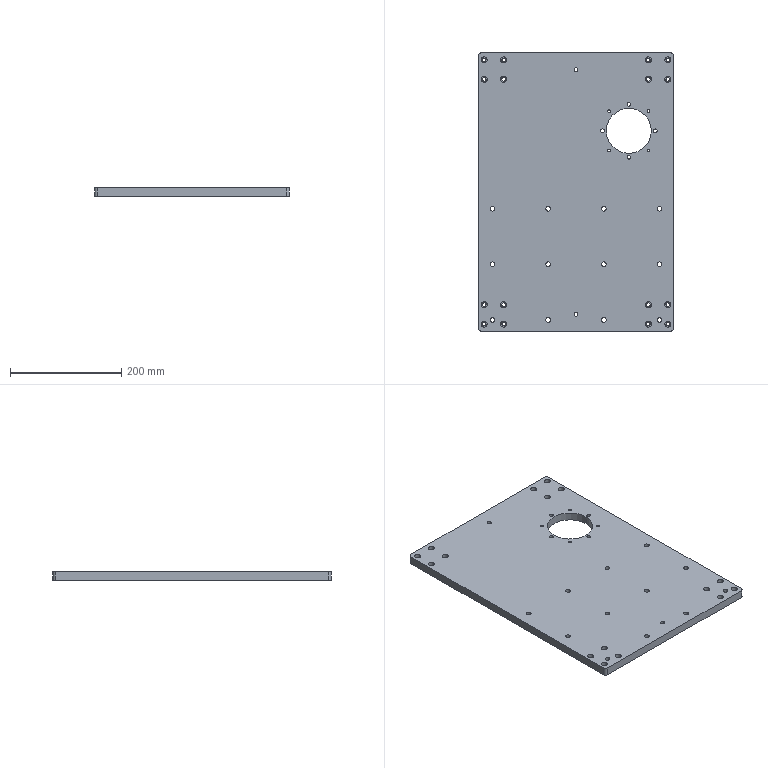NC program | Mastercam | posted with a generic post | part box 350 x 500 x 15 mm
Lines 1451 to 2012 of 4195:
N4600 T6 M6
N4610 G0 G90 G17 G54 X-110. Y-47.5 A0. S7000 M3
N4620 G43 H6 Z50. M8
N4630 Z1.
N4640 G1 Z0. F600.
N4650 X-111.711 Y-47.771 F3000.
N4660 G3 X-111.945 Y-48.491 I.991 J-.72
N4670 X-111.44 Y-49.482 I1.225 J0.
N4680 X-110. Y-49.95 Z-.05 I1.44 J1.982
N4690 X-107.55 Y-47.5 Z-.175 I0. J2.45
N4700 X-110. Y-45.05 Z-.3 I-2.45 J0.
N4710 X-112.45 Y-47.5 Z-.425 I0. J-2.45
N4720 X-111.44 Y-49.482 Z-.5 I2.45 J0.
N4730 X-110. Y-49.95 Z-.55 I1.44 J1.982
N4740 X-107.55 Y-47.5 Z-.675 I0. J2.45
N4750 X-110. Y-45.05 Z-.8 I-2.45 J0.
N4760 X-112.45 Y-47.5 Z-.925 I0. J-2.45
N4770 X-111.44 Y-49.482 Z-1. I2.45 J0.
N4780 X-110. Y-49.95 Z-1.05 I1.44 J1.982
N4790 X-107.55 Y-47.5 Z-1.175 I0. J2.45
N4800 X-110. Y-45.05 Z-1.3 I-2.45 J0.
N4810 X-112.45 Y-47.5 Z-1.425 I0. J-2.45
N4820 X-111.44 Y-49.482 Z-1.5 I2.45 J0.
N4830 X-110. Y-49.95 Z-1.55 I1.44 J1.982
N4840 X-107.55 Y-47.5 Z-1.675 I0. J2.45
N4850 X-110. Y-45.05 Z-1.8 I-2.45 J0.
N4860 X-112.45 Y-47.5 Z-1.925 I0. J-2.45
N4870 X-111.44 Y-49.482 Z-2. I2.45 J0.
N4880 X-110. Y-49.95 Z-2.05 I1.44 J1.982
N4890 X-107.55 Y-47.5 Z-2.175 I0. J2.45
N4900 X-110. Y-45.05 Z-2.3 I-2.45 J0.
N4910 X-112.45 Y-47.5 Z-2.425 I0. J-2.45
N4920 X-111.44 Y-49.482 Z-2.5 I2.45 J0.
N4930 X-110. Y-49.95 Z-2.55 I1.44 J1.982
N4940 X-107.55 Y-47.5 Z-2.675 I0. J2.45
N4950 X-110. Y-45.05 Z-2.8 I-2.45 J0.
N4960 X-112.45 Y-47.5 Z-2.925 I0. J-2.45
N4970 X-111.44 Y-49.482 Z-3. I2.45 J0.
N4980 X-110. Y-49.95 Z-3.05 I1.44 J1.982
N4990 X-107.55 Y-47.5 Z-3.175 I0. J2.45
N5000 X-110. Y-45.05 Z-3.3 I-2.45 J0.
N5010 X-112.45 Y-47.5 Z-3.425 I0. J-2.45
N5020 X-111.44 Y-49.482 Z-3.5 I2.45 J0.
N5030 X-110. Y-49.95 Z-3.55 I1.44 J1.982
N5040 X-107.55 Y-47.5 Z-3.675 I0. J2.45
N5050 X-110. Y-45.05 Z-3.8 I-2.45 J0.
N5060 X-112.45 Y-47.5 Z-3.925 I0. J-2.45
N5070 X-111.44 Y-49.482 Z-4. I2.45 J0.
N5080 X-110. Y-49.95 Z-4.05 I1.44 J1.982
N5090 X-107.55 Y-47.5 Z-4.175 I0. J2.45
N5100 X-110. Y-45.05 Z-4.3 I-2.45 J0.
N5110 X-112.45 Y-47.5 Z-4.425 I0. J-2.45
N5120 X-111.44 Y-49.482 Z-4.5 I2.45 J0.
N5130 X-110. Y-49.95 Z-4.55 I1.44 J1.982
N5140 X-107.55 Y-47.5 Z-4.675 I0. J2.45
N5150 X-110. Y-45.05 Z-4.8 I-2.45 J0.
N5160 X-112.45 Y-47.5 Z-4.925 I0. J-2.45
N5170 X-111.44 Y-49.482 Z-5. I2.45 J0.
N5180 X-110. Y-49.95 Z-5.05 I1.44 J1.982
N5190 X-107.55 Y-47.5 Z-5.175 I0. J2.45
N5200 X-110. Y-45.05 Z-5.3 I-2.45 J0.
N5210 X-112.45 Y-47.5 Z-5.425 I0. J-2.45
N5220 X-111.44 Y-49.482 Z-5.5 I2.45 J0.
N5230 X-110. Y-49.95 Z-5.55 I1.44 J1.982
N5240 X-107.55 Y-47.5 Z-5.675 I0. J2.45
N5250 X-110. Y-45.05 Z-5.8 I-2.45 J0.
N5260 X-112.45 Y-47.5 Z-5.925 I0. J-2.45
N5270 X-111.44 Y-49.482 Z-6. I2.45 J0.
N5280 X-110. Y-49.95 Z-6.05 I1.44 J1.982
N5290 X-107.55 Y-47.5 Z-6.175 I0. J2.45
N5300 X-110. Y-45.05 Z-6.3 I-2.45 J0.
N5310 X-112.45 Y-47.5 Z-6.425 I0. J-2.45
N5320 X-111.44 Y-49.482 Z-6.5 I2.45 J0.
N5330 X-110. Y-49.95 Z-6.55 I1.44 J1.982
N5340 X-107.55 Y-47.5 Z-6.675 I0. J2.45
N5350 X-110. Y-45.05 Z-6.8 I-2.45 J0.
N5360 X-112.45 Y-47.5 I0. J-2.45 F1500.
N5370 X-110. Y-49.95 I2.45 J0.
N5380 X-107.55 Y-47.5 I0. J2.45
N5390 X-110. Y-45.05 I-2.45 J0.
N5400 X-111.225 Y-46.275 I0. J-1.225
N5410 G1 X-110. Y-47.5
N5420 G0 Z0.
N5430 G1 X-108.75 Y-46.25 F750.
N5440 G3 X-110. Y-45. I-1.25 J0.
N5450 X-112.5 Y-47.5 I0. J-2.5
N5460 X-110. Y-50. I2.5 J0.
N5470 X-107.5 Y-47.5 I0. J2.5
N5480 X-110. Y-45. I-2.5 J0.
N5490 X-112.5 Y-47.5 Z-.5 I0. J-2.5
N5500 X-110. Y-50. Z-1. I2.5 J0.
N5510 X-107.5 Y-47.5 Z-1.5 I0. J2.5
N5520 X-110. Y-45. Z-2. I-2.5 J0.
N5530 X-112.5 Y-47.5 Z-2.5 I0. J-2.5
N5540 X-110. Y-50. Z-3. I2.5 J0.
N5550 X-107.5 Y-47.5 Z-3.5 I0. J2.5
N5560 X-110. Y-45. Z-4. I-2.5 J0.
N5570 X-112.5 Y-47.5 Z-4.5 I0. J-2.5
N5580 X-110. Y-50. Z-5. I2.5 J0.
N5590 X-107.5 Y-47.5 Z-5.5 I0. J2.5
N5600 X-110. Y-45. Z-6. I-2.5 J0.
N5610 X-112.5 Y-47.5 Z-6.5 I0. J-2.5
N5620 X-111.469 Y-49.523 Z-6.8 I2.5 J0.
N5630 X-110. Y-50. I1.469 J2.023
N5640 X-107.5 Y-47.5 I0. J2.5
N5650 X-110. Y-45. I-2.5 J0.
N5660 X-112.5 Y-47.5 I0. J-2.5
N5670 X-111.469 Y-49.523 I2.5 J0.
N5680 X-110.735 Y-49.761 I.734 J1.012
N5690 X-109.723 Y-49.246 I0. J1.25
N5700 G1 X-110. Y-47.5
N5710 G0 Z50.
N5720 X-157.5 Y-95.
N5730 Z1.
N5740 G1 Z0. F600.
N5750 X-159.211 Y-95.271 F3000.
N5760 G3 X-159.445 Y-95.991 I.991 J-.72
N5770 X-158.94 Y-96.982 I1.225 J0.
N5780 X-157.5 Y-97.45 Z-.05 I1.44 J1.982
N5790 X-155.05 Y-95. Z-.175 I0. J2.45
N5800 X-157.5 Y-92.55 Z-.3 I-2.45 J0.
N5810 X-159.95 Y-95. Z-.425 I0. J-2.45
N5820 X-158.94 Y-96.982 Z-.5 I2.45 J0.
N5830 X-157.5 Y-97.45 Z-.55 I1.44 J1.982
N5840 X-155.05 Y-95. Z-.675 I0. J2.45
N5850 X-157.5 Y-92.55 Z-.8 I-2.45 J0.
N5860 X-159.95 Y-95. Z-.925 I0. J-2.45
N5870 X-158.94 Y-96.982 Z-1. I2.45 J0.
N5880 X-157.5 Y-97.45 Z-1.05 I1.44 J1.982
N5890 X-155.05 Y-95. Z-1.175 I0. J2.45
N5900 X-157.5 Y-92.55 Z-1.3 I-2.45 J0.
N5910 X-159.95 Y-95. Z-1.425 I0. J-2.45
N5920 X-158.94 Y-96.982 Z-1.5 I2.45 J0.
N5930 X-157.5 Y-97.45 Z-1.55 I1.44 J1.982
N5940 X-155.05 Y-95. Z-1.675 I0. J2.45
N5950 X-157.5 Y-92.55 Z-1.8 I-2.45 J0.
N5960 X-159.95 Y-95. Z-1.925 I0. J-2.45
N5970 X-158.94 Y-96.982 Z-2. I2.45 J0.
N5980 X-157.5 Y-97.45 Z-2.05 I1.44 J1.982
N5990 X-155.05 Y-95. Z-2.175 I0. J2.45
N6000 X-157.5 Y-92.55 Z-2.3 I-2.45 J0.
N6010 X-159.95 Y-95. Z-2.425 I0. J-2.45
N6020 X-158.94 Y-96.982 Z-2.5 I2.45 J0.
N6030 X-157.5 Y-97.45 Z-2.55 I1.44 J1.982
N6040 X-155.05 Y-95. Z-2.675 I0. J2.45
N6050 X-157.5 Y-92.55 Z-2.8 I-2.45 J0.
N6060 X-159.95 Y-95. Z-2.925 I0. J-2.45
N6070 X-158.94 Y-96.982 Z-3. I2.45 J0.
N6080 X-157.5 Y-97.45 Z-3.05 I1.44 J1.982
N6090 X-155.05 Y-95. Z-3.175 I0. J2.45
N6100 X-157.5 Y-92.55 Z-3.3 I-2.45 J0.
N6110 X-159.95 Y-95. Z-3.425 I0. J-2.45
N6120 X-158.94 Y-96.982 Z-3.5 I2.45 J0.
N6130 X-157.5 Y-97.45 Z-3.55 I1.44 J1.982
N6140 X-155.05 Y-95. Z-3.675 I0. J2.45
N6150 X-157.5 Y-92.55 Z-3.8 I-2.45 J0.
N6160 X-159.95 Y-95. Z-3.925 I0. J-2.45
N6170 X-158.94 Y-96.982 Z-4. I2.45 J0.
N6180 X-157.5 Y-97.45 Z-4.05 I1.44 J1.982
N6190 X-155.05 Y-95. Z-4.175 I0. J2.45
N6200 X-157.5 Y-92.55 Z-4.3 I-2.45 J0.
N6210 X-159.95 Y-95. Z-4.425 I0. J-2.45
N6220 X-158.94 Y-96.982 Z-4.5 I2.45 J0.
N6230 X-157.5 Y-97.45 Z-4.55 I1.44 J1.982
N6240 X-155.05 Y-95. Z-4.675 I0. J2.45
N6250 X-157.5 Y-92.55 Z-4.8 I-2.45 J0.
N6260 X-159.95 Y-95. Z-4.925 I0. J-2.45
N6270 X-158.94 Y-96.982 Z-5. I2.45 J0.
N6280 X-157.5 Y-97.45 Z-5.05 I1.44 J1.982
N6290 X-155.05 Y-95. Z-5.175 I0. J2.45
N6300 X-157.5 Y-92.55 Z-5.3 I-2.45 J0.
N6310 X-159.95 Y-95. Z-5.425 I0. J-2.45
N6320 X-158.94 Y-96.982 Z-5.5 I2.45 J0.
N6330 X-157.5 Y-97.45 Z-5.55 I1.44 J1.982
N6340 X-155.05 Y-95. Z-5.675 I0. J2.45
N6350 X-157.5 Y-92.55 Z-5.8 I-2.45 J0.
N6360 X-159.95 Y-95. Z-5.925 I0. J-2.45
N6370 X-158.94 Y-96.982 Z-6. I2.45 J0.
N6380 X-157.5 Y-97.45 Z-6.05 I1.44 J1.982
N6390 X-155.05 Y-95. Z-6.175 I0. J2.45
N6400 X-157.5 Y-92.55 Z-6.3 I-2.45 J0.
N6410 X-159.95 Y-95. Z-6.425 I0. J-2.45
N6420 X-158.94 Y-96.982 Z-6.5 I2.45 J0.
N6430 X-157.5 Y-97.45 Z-6.55 I1.44 J1.982
N6440 X-155.05 Y-95. Z-6.675 I0. J2.45
N6450 X-157.5 Y-92.55 Z-6.8 I-2.45 J0.
N6460 X-159.95 Y-95. I0. J-2.45 F1500.
N6470 X-157.5 Y-97.45 I2.45 J0.
N6480 X-155.05 Y-95. I0. J2.45
N6490 X-157.5 Y-92.55 I-2.45 J0.
N6500 X-158.725 Y-93.775 I0. J-1.225
N6510 G1 X-157.5 Y-95.
N6520 G0 Z0.
N6530 G1 X-156.25 Y-93.75 F750.
N6540 G3 X-157.5 Y-92.5 I-1.25 J0.
N6550 X-160. Y-95. I0. J-2.5
N6560 X-157.5 Y-97.5 I2.5 J0.
N6570 X-155. Y-95. I0. J2.5
N6580 X-157.5 Y-92.5 I-2.5 J0.
N6590 X-160. Y-95. Z-.5 I0. J-2.5
N6600 X-157.5 Y-97.5 Z-1. I2.5 J0.
N6610 X-155. Y-95. Z-1.5 I0. J2.5
N6620 X-157.5 Y-92.5 Z-2. I-2.5 J0.
N6630 X-160. Y-95. Z-2.5 I0. J-2.5
N6640 X-157.5 Y-97.5 Z-3. I2.5 J0.
N6650 X-155. Y-95. Z-3.5 I0. J2.5
N6660 X-157.5 Y-92.5 Z-4. I-2.5 J0.
N6670 X-160. Y-95. Z-4.5 I0. J-2.5
N6680 X-157.5 Y-97.5 Z-5. I2.5 J0.
N6690 X-155. Y-95. Z-5.5 I0. J2.5
N6700 X-157.5 Y-92.5 Z-6. I-2.5 J0.
N6710 X-160. Y-95. Z-6.5 I0. J-2.5
N6720 X-158.969 Y-97.023 Z-6.8 I2.5 J0.
N6730 X-157.5 Y-97.5 I1.469 J2.023
N6740 X-155. Y-95. I0. J2.5
N6750 X-157.5 Y-92.5 I-2.5 J0.
N6760 X-160. Y-95. I0. J-2.5
N6770 X-158.969 Y-97.023 I2.5 J0.
N6780 X-158.235 Y-97.261 I.734 J1.012
N6790 X-157.223 Y-96.746 I0. J1.25
N6800 G1 X-157.5 Y-95.
N6810 G0 Z50.
N6820 X-110. Y-142.5
N6830 Z1.
N6840 G1 Z0. F600.
N6850 X-111.711 Y-142.771 F3000.
N6860 G3 X-111.945 Y-143.491 I.991 J-.72
N6870 X-111.44 Y-144.482 I1.225 J0.
N6880 X-110. Y-144.95 Z-.05 I1.44 J1.982
N6890 X-107.55 Y-142.5 Z-.175 I0. J2.45
N6900 X-110. Y-140.05 Z-.3 I-2.45 J0.
N6910 X-112.45 Y-142.5 Z-.425 I0. J-2.45
N6920 X-111.44 Y-144.482 Z-.5 I2.45 J0.
N6930 X-110. Y-144.95 Z-.55 I1.44 J1.982
N6940 X-107.55 Y-142.5 Z-.675 I0. J2.45
N6950 X-110. Y-140.05 Z-.8 I-2.45 J0.
N6960 X-112.45 Y-142.5 Z-.925 I0. J-2.45
N6970 X-111.44 Y-144.482 Z-1. I2.45 J0.
N6980 X-110. Y-144.95 Z-1.05 I1.44 J1.982
N6990 X-107.55 Y-142.5 Z-1.175 I0. J2.45
N7000 X-110. Y-140.05 Z-1.3 I-2.45 J0.
N7010 X-112.45 Y-142.5 Z-1.425 I0. J-2.45
N7020 X-111.44 Y-144.482 Z-1.5 I2.45 J0.
N7030 X-110. Y-144.95 Z-1.55 I1.44 J1.982
N7040 X-107.55 Y-142.5 Z-1.675 I0. J2.45
N7050 X-110. Y-140.05 Z-1.8 I-2.45 J0.
N7060 X-112.45 Y-142.5 Z-1.925 I0. J-2.45
N7070 X-111.44 Y-144.482 Z-2. I2.45 J0.
N7080 X-110. Y-144.95 Z-2.05 I1.44 J1.982
N7090 X-107.55 Y-142.5 Z-2.175 I0. J2.45
N7100 X-110. Y-140.05 Z-2.3 I-2.45 J0.
N7110 X-112.45 Y-142.5 Z-2.425 I0. J-2.45
N7120 X-111.44 Y-144.482 Z-2.5 I2.45 J0.
N7130 X-110. Y-144.95 Z-2.55 I1.44 J1.982
N7140 X-107.55 Y-142.5 Z-2.675 I0. J2.45
N7150 X-110. Y-140.05 Z-2.8 I-2.45 J0.
N7160 X-112.45 Y-142.5 Z-2.925 I0. J-2.45
N7170 X-111.44 Y-144.482 Z-3. I2.45 J0.
N7180 X-110. Y-144.95 Z-3.05 I1.44 J1.982
N7190 X-107.55 Y-142.5 Z-3.175 I0. J2.45
N7200 X-110. Y-140.05 Z-3.3 I-2.45 J0.
N7210 X-112.45 Y-142.5 Z-3.425 I0. J-2.45
N7220 X-111.44 Y-144.482 Z-3.5 I2.45 J0.
N7230 X-110. Y-144.95 Z-3.55 I1.44 J1.982
N7240 X-107.55 Y-142.5 Z-3.675 I0. J2.45
N7250 X-110. Y-140.05 Z-3.8 I-2.45 J0.
N7260 X-112.45 Y-142.5 Z-3.925 I0. J-2.45
N7270 X-111.44 Y-144.482 Z-4. I2.45 J0.
N7280 X-110. Y-144.95 Z-4.05 I1.44 J1.982
N7290 X-107.55 Y-142.5 Z-4.175 I0. J2.45
N7300 X-110. Y-140.05 Z-4.3 I-2.45 J0.
N7310 X-112.45 Y-142.5 Z-4.425 I0. J-2.45
N7320 X-111.44 Y-144.482 Z-4.5 I2.45 J0.
N7330 X-110. Y-144.95 Z-4.55 I1.44 J1.982
N7340 X-107.55 Y-142.5 Z-4.675 I0. J2.45
N7350 X-110. Y-140.05 Z-4.8 I-2.45 J0.
N7360 X-112.45 Y-142.5 Z-4.925 I0. J-2.45
N7370 X-111.44 Y-144.482 Z-5. I2.45 J0.
N7380 X-110. Y-144.95 Z-5.05 I1.44 J1.982
N7390 X-107.55 Y-142.5 Z-5.175 I0. J2.45
N7400 X-110. Y-140.05 Z-5.3 I-2.45 J0.
N7410 X-112.45 Y-142.5 Z-5.425 I0. J-2.45
N7420 X-111.44 Y-144.482 Z-5.5 I2.45 J0.
N7430 X-110. Y-144.95 Z-5.55 I1.44 J1.982
N7440 X-107.55 Y-142.5 Z-5.675 I0. J2.45
N7450 X-110. Y-140.05 Z-5.8 I-2.45 J0.
N7460 X-112.45 Y-142.5 Z-5.925 I0. J-2.45
N7470 X-111.44 Y-144.482 Z-6. I2.45 J0.
N7480 X-110. Y-144.95 Z-6.05 I1.44 J1.982
N7490 X-107.55 Y-142.5 Z-6.175 I0. J2.45
N7500 X-110. Y-140.05 Z-6.3 I-2.45 J0.
N7510 X-112.45 Y-142.5 Z-6.425 I0. J-2.45
N7520 X-111.44 Y-144.482 Z-6.5 I2.45 J0.
N7530 X-110. Y-144.95 Z-6.55 I1.44 J1.982
N7540 X-107.55 Y-142.5 Z-6.675 I0. J2.45
N7550 X-110. Y-140.05 Z-6.8 I-2.45 J0.
N7560 X-112.45 Y-142.5 I0. J-2.45 F1500.
N7570 X-110. Y-144.95 I2.45 J0.
N7580 X-107.55 Y-142.5 I0. J2.45
N7590 X-110. Y-140.05 I-2.45 J0.
N7600 X-111.225 Y-141.275 I0. J-1.225
N7610 G1 X-110. Y-142.5
N7620 G0 Z0.
N7630 G1 X-108.75 Y-141.25 F750.
N7640 G3 X-110. Y-140. I-1.25 J0.
N7650 X-112.5 Y-142.5 I0. J-2.5
N7660 X-110. Y-145. I2.5 J0.
N7670 X-107.5 Y-142.5 I0. J2.5
N7680 X-110. Y-140. I-2.5 J0.
N7690 X-112.5 Y-142.5 Z-.5 I0. J-2.5
N7700 X-110. Y-145. Z-1. I2.5 J0.
N7710 X-107.5 Y-142.5 Z-1.5 I0. J2.5
N7720 X-110. Y-140. Z-2. I-2.5 J0.
N7730 X-112.5 Y-142.5 Z-2.5 I0. J-2.5
N7740 X-110. Y-145. Z-3. I2.5 J0.
N7750 X-107.5 Y-142.5 Z-3.5 I0. J2.5
N7760 X-110. Y-140. Z-4. I-2.5 J0.
N7770 X-112.5 Y-142.5 Z-4.5 I0. J-2.5
N7780 X-110. Y-145. Z-5. I2.5 J0.
N7790 X-107.5 Y-142.5 Z-5.5 I0. J2.5
N7800 X-110. Y-140. Z-6. I-2.5 J0.
N7810 X-112.5 Y-142.5 Z-6.5 I0. J-2.5
N7820 X-111.469 Y-144.523 Z-6.8 I2.5 J0.
N7830 X-110. Y-145. I1.469 J2.023
N7840 X-107.5 Y-142.5 I0. J2.5
N7850 X-110. Y-140. I-2.5 J0.
N7860 X-112.5 Y-142.5 I0. J-2.5
N7870 X-111.469 Y-144.523 I2.5 J0.
N7880 X-110.735 Y-144.761 I.734 J1.012
N7890 X-109.723 Y-144.246 I0. J1.25
N7900 G1 X-110. Y-142.5
N7910 G0 Z50.
N7920 X-62.5 Y-95.
N7930 Z1.
N7940 G1 Z0. F600.
N7950 X-64.211 Y-95.271 F3000.
N7960 G3 X-64.445 Y-95.991 I.991 J-.72
N7970 X-63.94 Y-96.982 I1.225 J0.
N7980 X-62.5 Y-97.45 Z-.05 I1.44 J1.982
N7990 X-60.05 Y-95. Z-.175 I0. J2.45
N8000 X-62.5 Y-92.55 Z-.3 I-2.45 J0.
N8010 X-64.95 Y-95. Z-.425 I0. J-2.45
N8020 X-63.94 Y-96.982 Z-.5 I2.45 J0.
N8030 X-62.5 Y-97.45 Z-.55 I1.44 J1.982
N8040 X-60.05 Y-95. Z-.675 I0. J2.45
N8050 X-62.5 Y-92.55 Z-.8 I-2.45 J0.
N8060 X-64.95 Y-95. Z-.925 I0. J-2.45
N8070 X-63.94 Y-96.982 Z-1. I2.45 J0.
N8080 X-62.5 Y-97.45 Z-1.05 I1.44 J1.982
N8090 X-60.05 Y-95. Z-1.175 I0. J2.45
N8100 X-62.5 Y-92.55 Z-1.3 I-2.45 J0.
N8110 X-64.95 Y-95. Z-1.425 I0. J-2.45
N8120 X-63.94 Y-96.982 Z-1.5 I2.45 J0.
N8130 X-62.5 Y-97.45 Z-1.55 I1.44 J1.982
N8140 X-60.05 Y-95. Z-1.675 I0. J2.45
N8150 X-62.5 Y-92.55 Z-1.8 I-2.45 J0.
N8160 X-64.95 Y-95. Z-1.925 I0. J-2.45
N8170 X-63.94 Y-96.982 Z-2. I2.45 J0.
N8180 X-62.5 Y-97.45 Z-2.05 I1.44 J1.982
N8190 X-60.05 Y-95. Z-2.175 I0. J2.45
N8200 X-62.5 Y-92.55 Z-2.3 I-2.45 J0.
N8210 X-64.95 Y-95. Z-2.425 I0. J-2.45
N8220 X-63.94 Y-96.982 Z-2.5 I2.45 J0.
N8230 X-62.5 Y-97.45 Z-2.55 I1.44 J1.982
N8240 X-60.05 Y-95. Z-2.675 I0. J2.45
N8250 X-62.5 Y-92.55 Z-2.8 I-2.45 J0.
N8260 X-64.95 Y-95. Z-2.925 I0. J-2.45
N8270 X-63.94 Y-96.982 Z-3. I2.45 J0.
N8280 X-62.5 Y-97.45 Z-3.05 I1.44 J1.982
N8290 X-60.05 Y-95. Z-3.175 I0. J2.45
N8300 X-62.5 Y-92.55 Z-3.3 I-2.45 J0.
N8310 X-64.95 Y-95. Z-3.425 I0. J-2.45
N8320 X-63.94 Y-96.982 Z-3.5 I2.45 J0.
N8330 X-62.5 Y-97.45 Z-3.55 I1.44 J1.982
N8340 X-60.05 Y-95. Z-3.675 I0. J2.45
N8350 X-62.5 Y-92.55 Z-3.8 I-2.45 J0.
N8360 X-64.95 Y-95. Z-3.925 I0. J-2.45
N8370 X-63.94 Y-96.982 Z-4. I2.45 J0.
N8380 X-62.5 Y-97.45 Z-4.05 I1.44 J1.982
N8390 X-60.05 Y-95. Z-4.175 I0. J2.45
N8400 X-62.5 Y-92.55 Z-4.3 I-2.45 J0.
N8410 X-64.95 Y-95. Z-4.425 I0. J-2.45
N8420 X-63.94 Y-96.982 Z-4.5 I2.45 J0.
N8430 X-62.5 Y-97.45 Z-4.55 I1.44 J1.982
N8440 X-60.05 Y-95. Z-4.675 I0. J2.45
N8450 X-62.5 Y-92.55 Z-4.8 I-2.45 J0.
N8460 X-64.95 Y-95. Z-4.925 I0. J-2.45
N8470 X-63.94 Y-96.982 Z-5. I2.45 J0.
N8480 X-62.5 Y-97.45 Z-5.05 I1.44 J1.982
N8490 X-60.05 Y-95. Z-5.175 I0. J2.45
N8500 X-62.5 Y-92.55 Z-5.3 I-2.45 J0.
N8510 X-64.95 Y-95. Z-5.425 I0. J-2.45
N8520 X-63.94 Y-96.982 Z-5.5 I2.45 J0.
N8530 X-62.5 Y-97.45 Z-5.55 I1.44 J1.982
N8540 X-60.05 Y-95. Z-5.675 I0. J2.45
N8550 X-62.5 Y-92.55 Z-5.8 I-2.45 J0.
N8560 X-64.95 Y-95. Z-5.925 I0. J-2.45
N8570 X-63.94 Y-96.982 Z-6. I2.45 J0.
N8580 X-62.5 Y-97.45 Z-6.05 I1.44 J1.982
N8590 X-60.05 Y-95. Z-6.175 I0. J2.45
N8600 X-62.5 Y-92.55 Z-6.3 I-2.45 J0.
N8610 X-64.95 Y-95. Z-6.425 I0. J-2.45
N8620 X-63.94 Y-96.982 Z-6.5 I2.45 J0.
N8630 X-62.5 Y-97.45 Z-6.55 I1.44 J1.982
N8640 X-60.05 Y-95. Z-6.675 I0. J2.45
N8650 X-62.5 Y-92.55 Z-6.8 I-2.45 J0.
N8660 X-64.95 Y-95. I0. J-2.45 F1500.
N8670 X-62.5 Y-97.45 I2.45 J0.
N8680 X-60.05 Y-95. I0. J2.45
N8690 X-62.5 Y-92.55 I-2.45 J0.
N8700 X-63.725 Y-93.775 I0. J-1.225
N8710 G1 X-62.5 Y-95.
N8720 G0 Z0.
N8730 G1 X-61.25 Y-93.75 F750.
N8740 G3 X-62.5 Y-92.5 I-1.25 J0.
N8750 X-65. Y-95. I0. J-2.5
N8760 X-62.5 Y-97.5 I2.5 J0.
N8770 X-60. Y-95. I0. J2.5
N8780 X-62.5 Y-92.5 I-2.5 J0.
N8790 X-65. Y-95. Z-.5 I0. J-2.5
N8800 X-62.5 Y-97.5 Z-1. I2.5 J0.
N8810 X-60. Y-95. Z-1.5 I0. J2.5
N8820 X-62.5 Y-92.5 Z-2. I-2.5 J0.
N8830 X-65. Y-95. Z-2.5 I0. J-2.5
N8840 X-62.5 Y-97.5 Z-3. I2.5 J0.
N8850 X-60. Y-95. Z-3.5 I0. J2.5
N8860 X-62.5 Y-92.5 Z-4. I-2.5 J0.
N8870 X-65. Y-95. Z-4.5 I0. J-2.5
N8880 X-62.5 Y-97.5 Z-5. I2.5 J0.
N8890 X-60. Y-95. Z-5.5 I0. J2.5
N8900 X-62.5 Y-92.5 Z-6. I-2.5 J0.
N8910 X-65. Y-95. Z-6.5 I0. J-2.5
N8920 X-63.969 Y-97.023 Z-6.8 I2.5 J0.
N8930 X-62.5 Y-97.5 I1.469 J2.023
N8940 X-60. Y-95. I0. J2.5
N8950 X-62.5 Y-92.5 I-2.5 J0.
N8960 X-65. Y-95. I0. J-2.5
N8970 X-63.969 Y-97.023 I2.5 J0.
N8980 X-63.235 Y-97.261 I.734 J1.012
N8990 X-62.223 Y-96.746 I0. J1.25
N9000 G1 X-62.5 Y-95.
N9010 G0 Z50.
N9020 M5
N9030 G91 G28 Z0. M9
N9040 A0.
N9050 M01
N9060 T7 M6
N9070 G0 G90 G17 G54 X30. Y-50. A0. S3000 M3
N9080 G43 H7 Z50. M8
N9090 G98 G81 Z-.7 R1. F300.
N9100 Y50.
N9110 X130.
N9120 Y-50.
N9130 X230.
N9140 X220. Y0.
N9150 X230. Y50.
N9160 X237.5 Y130.
N9170 X230. Y150.
N9180 X237.5 Y165.
N9190 X202.5
N9200 Y130.
N9210 X130. Y150.
N9220 X30.
N9230 X-202.5 Y165.
N9240 X-237.5
N9250 Y130.
N9260 X-202.5
N9270 X-220. Y0.
N9280 X-145.355 Y-59.645
N9290 G80
N9300 G0
N9310 X-157.5 Y-95.
N9320 Z43.2
N9330 G98 G81 Z-7.5 R-5.8 F300.
N9340 G80
N9350 G0 Z50.
N9360 X-202.5 Y-130.
N9370 G98 G81 Z-.7 R1. F300.
N9380 X-237.5
N9390 Y-165.
N9400 X-202.5
N9410 X-145.355 Y-130.355
N9420 G80
N9430 G0
N9440 X-110. Y-142.5
N9450 Z43.2
N9460 G98 G81 Z-7.5 R-5.8 F300.
N9470 Y-47.5
N9480 G80
N9490 G0 Z50.
N9500 X-74.645 Y-59.645
N9510 G98 G81 Z-.7 R1. F300.
N9520 G80
N9530 G0
N9540 X-62.5 Y-95.
N9550 Z43.2
N9560 G98 G81 Z-7.5 R-5.8 F300.
N9570 G80
N9580 G0 Z50.
N9590 X-74.645 Y-130.355
N9600 G98 G81 Z-.7 R1. F300.
N9610 X30. Y-150.
N9620 X130.
N9630 X202.5 Y-165.
N9640 X237.5
N9650 X230. Y-150.
N9660 X237.5 Y-130.
N9670 X202.5
N9680 G80
N9690 S7000 M3
N9700 G0 X-109.6 Y-43.45
N9710 Z1.
N9720 G1 Z-.8 F600.
N9730 Y-43.05 F1000.
N9740 G3 X-110. Y-42.65 I-.4 J0.
N9750 X-114.85 Y-47.5 I0. J-4.85
N9760 X-110. Y-52.35 I4.85 J0.
N9770 X-105.15 Y-47.5 I0. J4.85
N9780 X-110. Y-42.65 I-4.85 J0.
N9790 X-110.4 Y-43.05 I0. J-.4
N9800 G1 Y-43.45
N9810 G0 Z50.
N9820 X-62.1 Y-90.95
N9830 Z1.
N9840 G1 Z-.8 F600.
N9850 Y-90.55 F1000.
N9860 G3 X-62.5 Y-90.15 I-.4 J0.
N9870 X-67.35 Y-95. I0. J-4.85
N9880 X-62.5 Y-99.85 I4.85 J0.
N9890 X-57.65 Y-95. I0. J4.85
N9900 X-62.5 Y-90.15 I-4.85 J0.
N9910 X-62.9 Y-90.55 I0. J-.4
N9920 G1 Y-90.95
N9930 G0 Z50.
N9940 X-109.6 Y-138.45
N9950 Z1.
N9960 G1 Z-.8 F600.
N9970 Y-138.05 F1000.
N9980 G3 X-110. Y-137.65 I-.4 J0.
N9990 X-114.85 Y-142.5 I0. J-4.85
N100 X-110. Y-147.35 I4.85 J0.
N110 X-105.15 Y-142.5 I0. J4.85
N120 X-110. Y-137.65 I-4.85 J0.
N130 X-110.4 Y-138.05 I0. J-.4
N140 G1 Y-138.45
N150 G0 Z50.
N160 X-157.1 Y-90.95
N170 Z1.
N180 G1 Z-.8 F600.
N190 Y-90.55 F1000.
N200 G3 X-157.5 Y-90.15 I-.4 J0.
N210 X-162.35 Y-95. I0. J-4.85
N220 X-157.5 Y-99.85 I4.85 J0.
N230 X-152.65 Y-95. I0. J4.85
N240 X-157.5 Y-90.15 I-4.85 J0.
N250 X-157.9 Y-90.55 I0. J-.4
N260 G1 Y-90.95
N270 G0 Z50.
N280 M5
N290 G91 G28 Z0. M9
N300 A0.
N310 M01